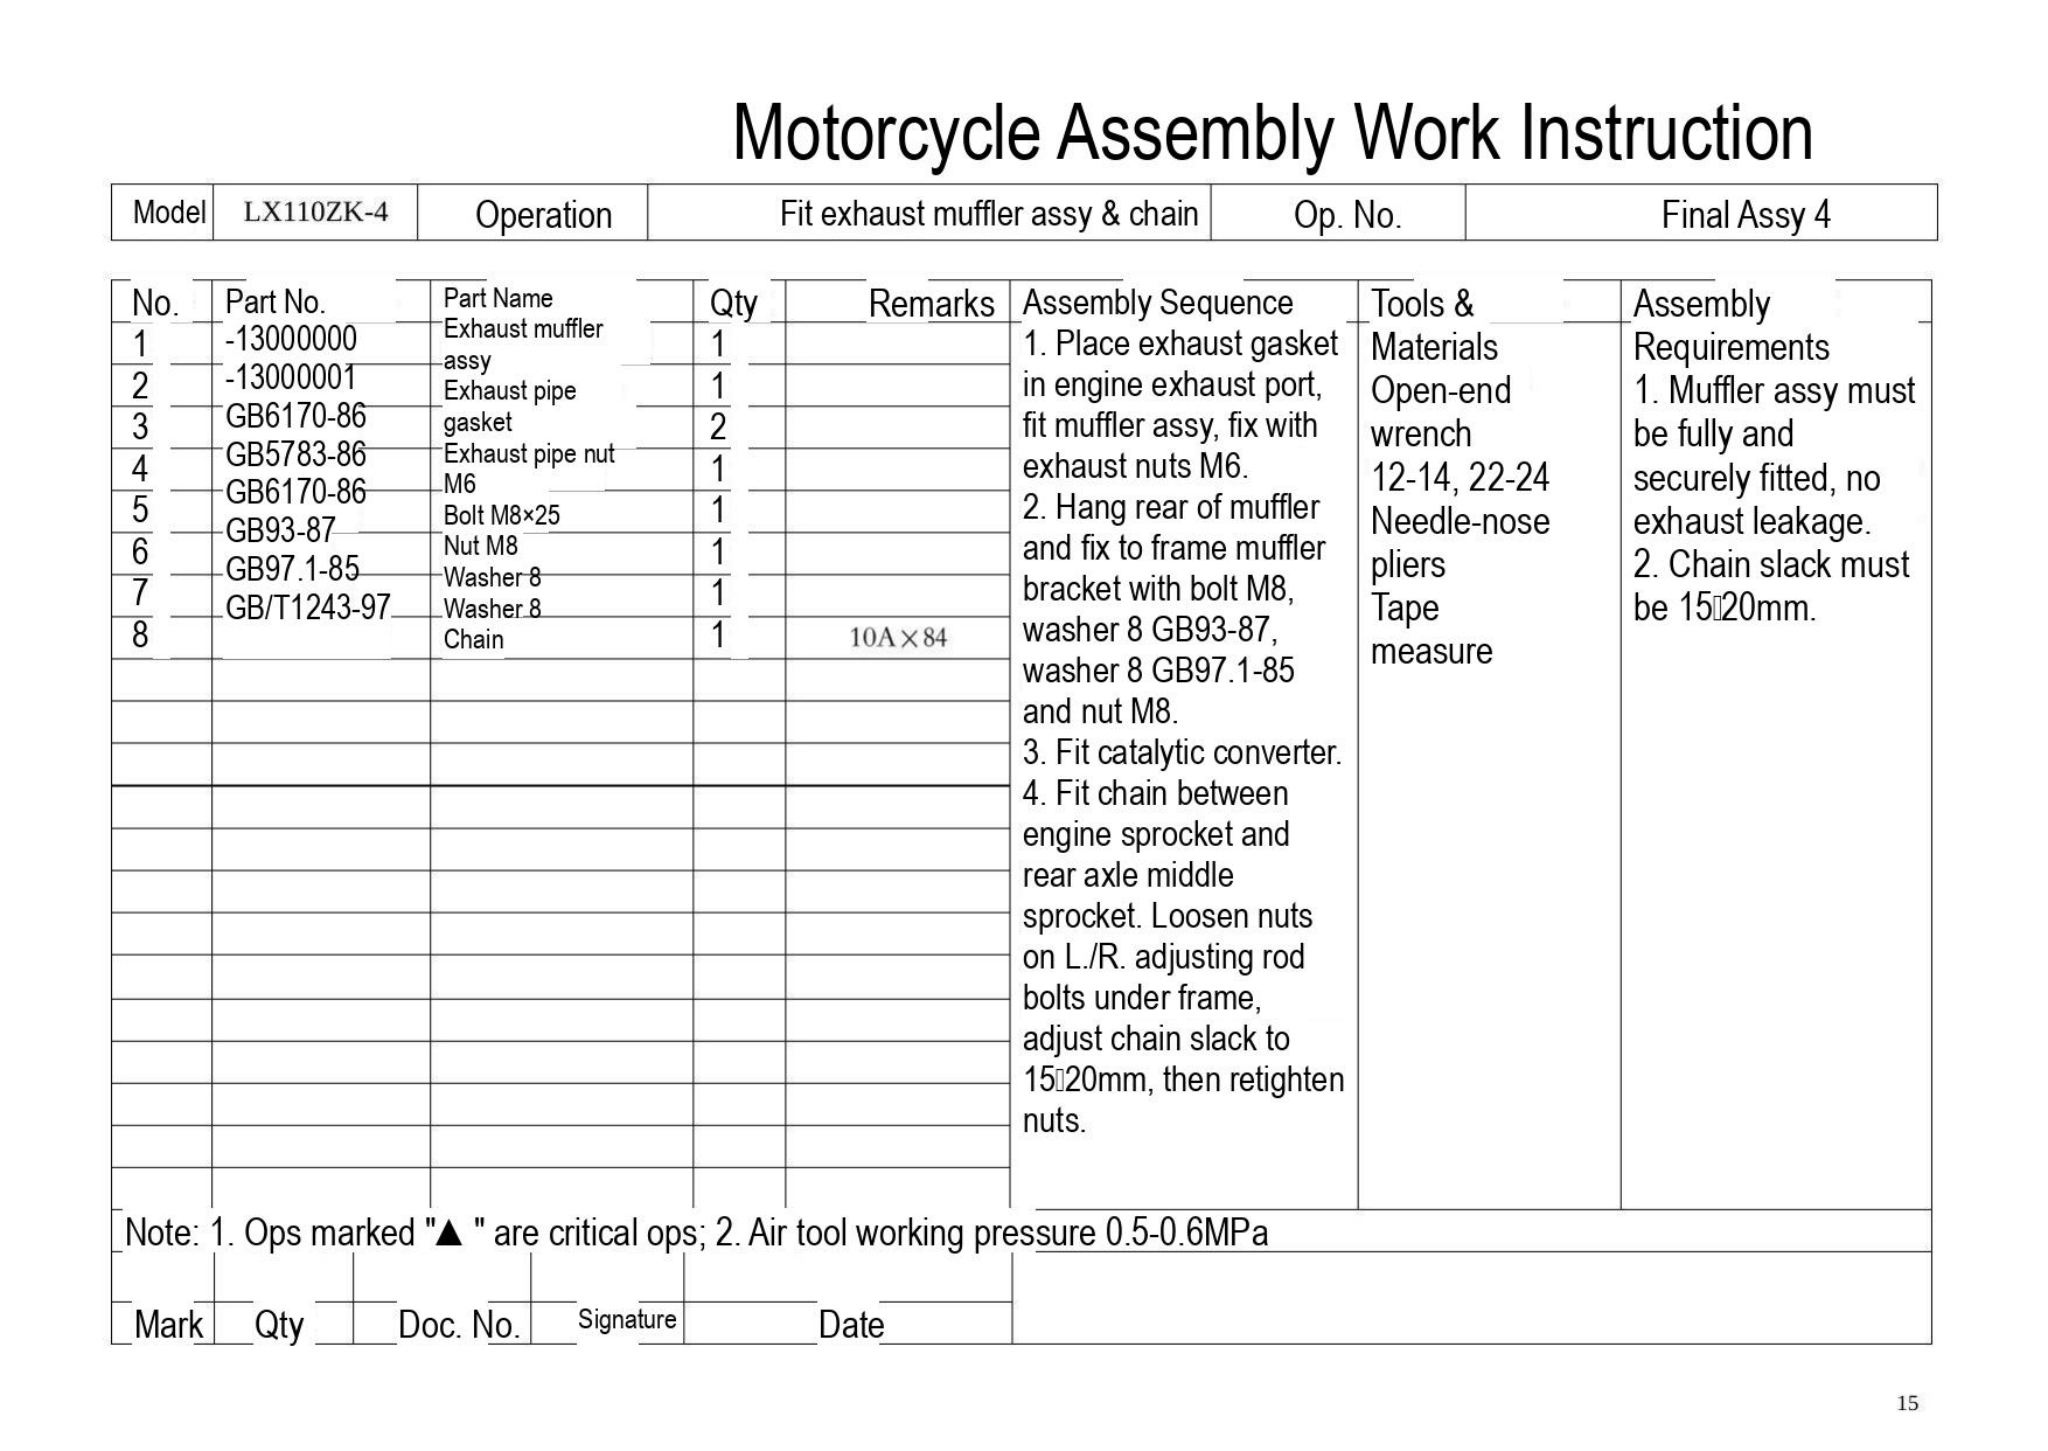# Motorcycle Assembly Work Instruction

| Model | LX110ZK-4 | Operation | Fit exhaust muffler assy & chain | Op. No. | Final Assy 4 |
|---|---|---|---|---|---|

| No. | Part No. | Part Name | Qty | Remarks |
|---|---|---|---|---|
| 1 | -13000000 | Exhaust muffler assy | 1 | |
| 2 | -13000001 | Exhaust pipe gasket | 1 | |
| 3 | GB6170-86 | Exhaust pipe nut M6 | 2 | |
| 4 | GB5783-86 | Bolt M8×25 | 1 | |
| 5 | GB6170-86 | Nut M8 | 1 | |
| 6 | GB93-87 | Washer 8 | 1 | |
| 7 | GB97.1-85 | Washer 8 | 1 | |
| 8 | GB/T1243-97 | Chain | 1 | 10A×84 |

| Assembly Sequence | Tools & Materials | Assembly Requirements |
|---|---|---|
| 1. Place exhaust gasket in engine exhaust port, fit muffler assy, fix with exhaust nuts M6.<br>2. Hang rear of muffler and fix to frame muffler bracket with bolt M8, washer 8 GB93-87, washer 8 GB97.1-85 and nut M8.<br>3. Fit catalytic converter.<br>4. Fit chain between engine sprocket and rear axle middle sprocket. Loosen nuts on L./R. adjusting rod bolts under frame, adjust chain slack to 15▯20mm, then retighten nuts. | Open-end wrench 12-14, 22-24<br>Needle-nose pliers<br>Tape measure | 1. Muffler assy must be fully and securely fitted, no exhaust leakage.<br>2. Chain slack must be 15▯20mm. |

Note: 1. Ops marked "▲ " are critical ops; 2. Air tool working pressure 0.5-0.6MPa

| Mark | Qty | Doc. No. | Signature | Date |
|---|---|---|---|---|

15
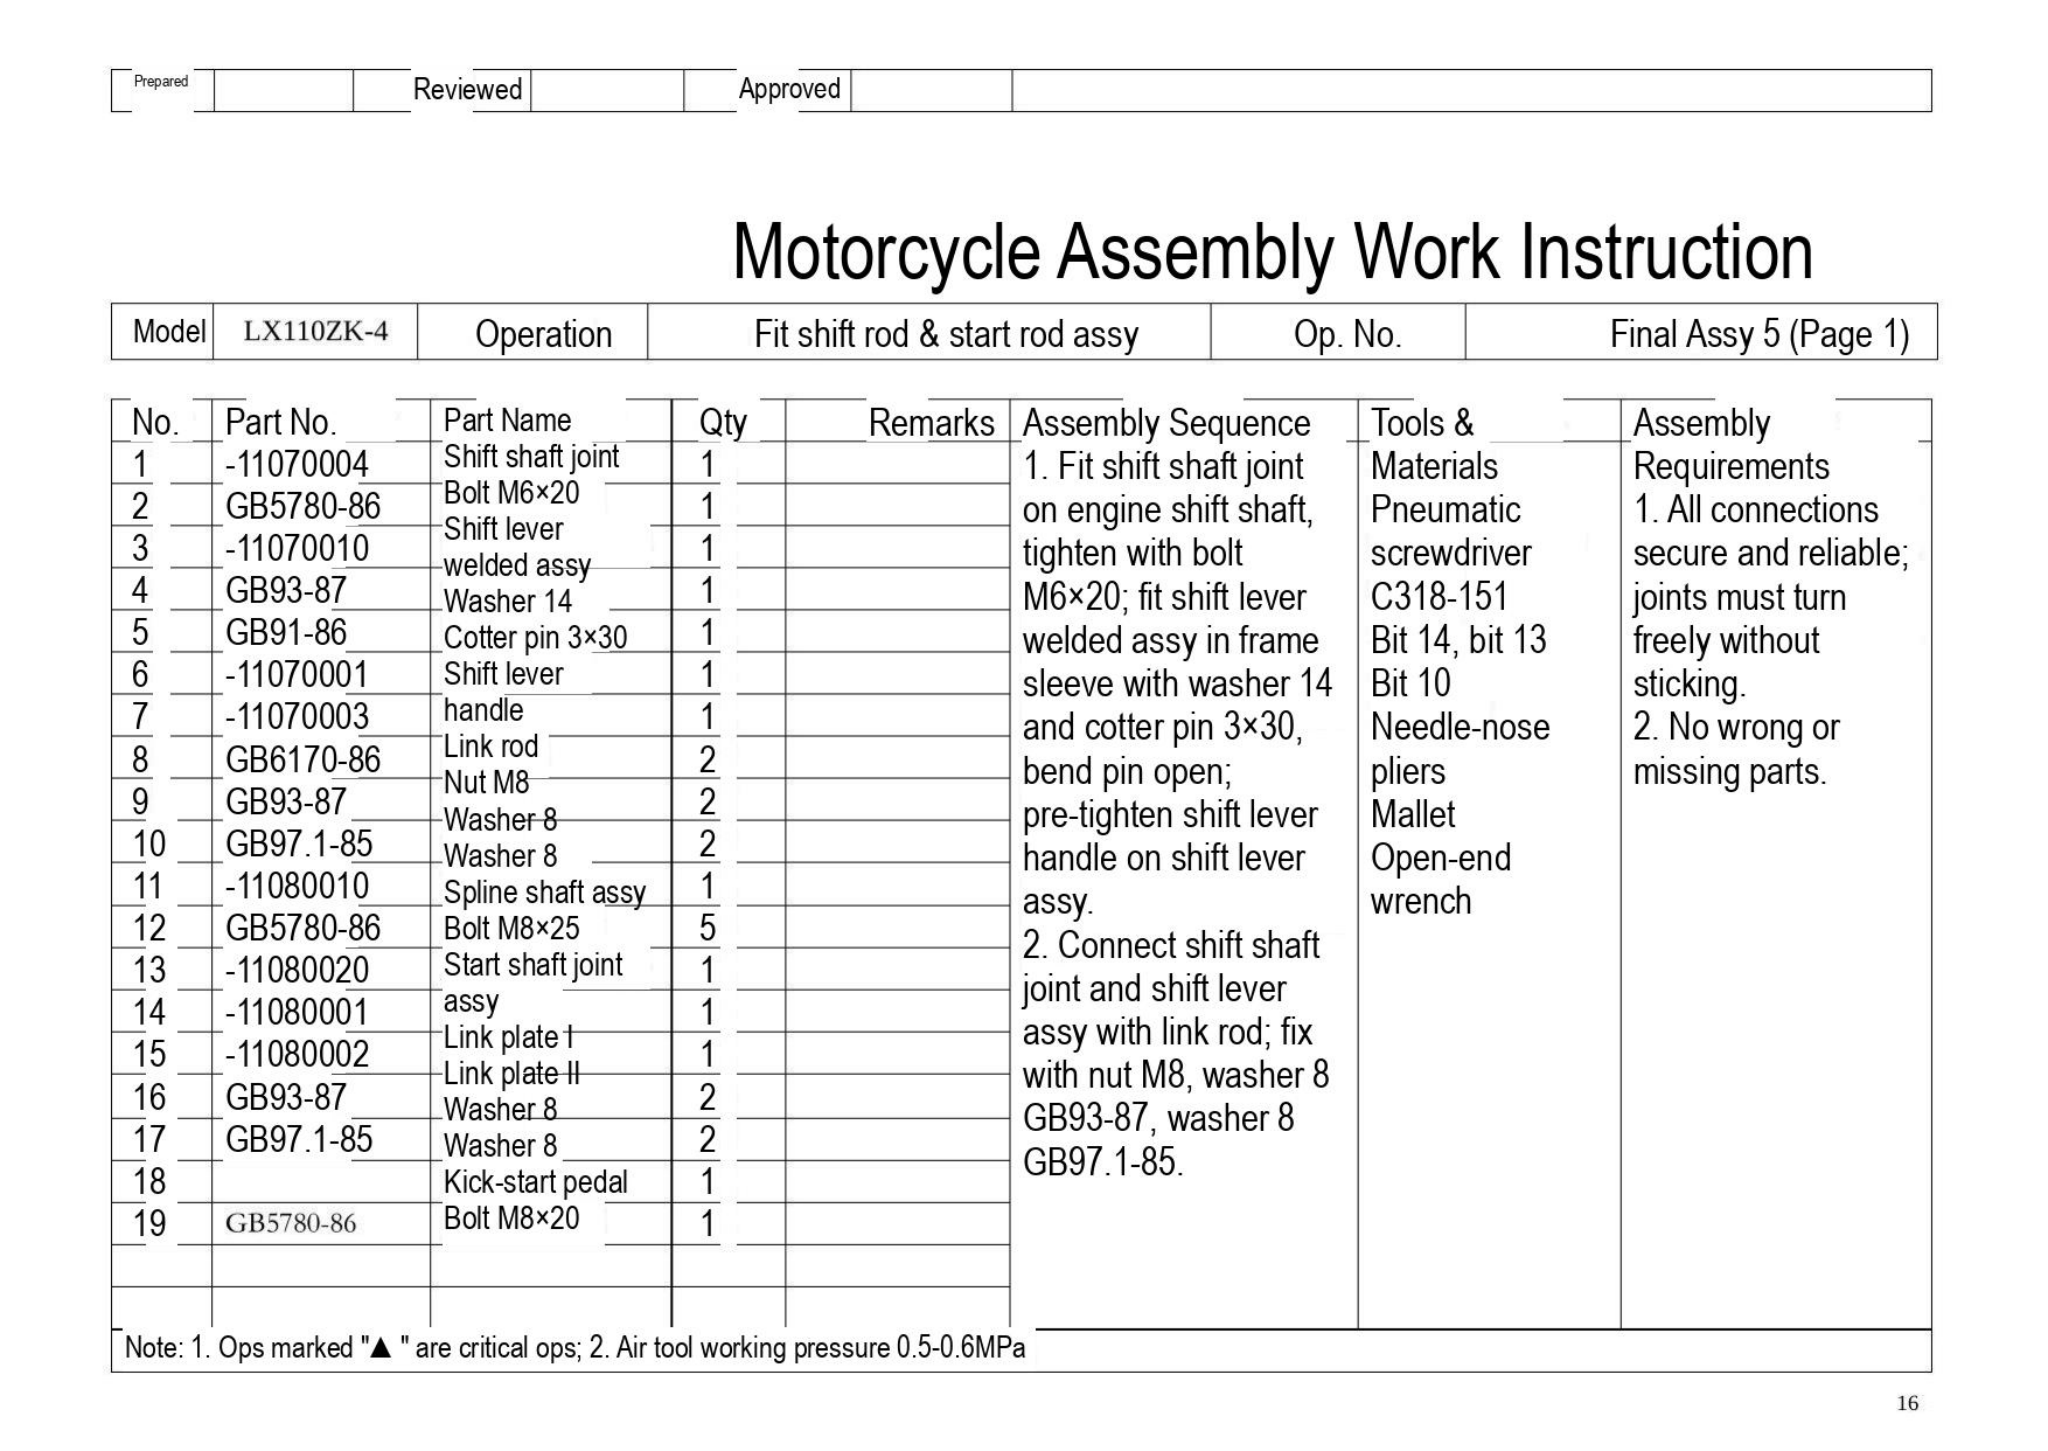| Prepared | | Reviewed | | Approved | | |
|---|---|---|---|---|---|---|

# Motorcycle Assembly Work Instruction

| Model | LX110ZK-4 | Operation | Fit shift rod & start rod assy | Op. No. | Final Assy 5 (Page 1) |
|---|---|---|---|---|---|

| No. | Part No. | Part Name | Qty | Remarks |
|---|---|---|---|---|
| 1 | -11070004 | Shift shaft joint | 1 | |
| 2 | GB5780-86 | Bolt M6×20 | 1 | |
| 3 | -11070010 | Shift lever welded assy | 1 | |
| 4 | GB93-87 | Washer 14 | 1 | |
| 5 | GB91-86 | Cotter pin 3×30 | 1 | |
| 6 | -11070001 | Shift lever handle | 1 | |
| 7 | -11070003 | Link rod | 1 | |
| 8 | GB6170-86 | Nut M8 | 2 | |
| 9 | GB93-87 | Washer 8 | 2 | |
| 10 | GB97.1-85 | Washer 8 | 2 | |
| 11 | -11080010 | Spline shaft assy | 1 | |
| 12 | GB5780-86 | Bolt M8×25 | 5 | |
| 13 | -11080020 | Start shaft joint assy | 1 | |
| 14 | -11080001 | Link plate I | 1 | |
| 15 | -11080002 | Link plate II | 1 | |
| 16 | GB93-87 | Washer 8 | 2 | |
| 17 | GB97.1-85 | Washer 8 | 2 | |
| 18 | | Kick-start pedal | 1 | |
| 19 | GB5780-86 | Bolt M8×20 | 1 | |
| | | | | |
| | | | | |

| Assembly Sequence | Tools & Materials | Assembly Requirements |
|---|---|---|
| 1. Fit shift shaft joint on engine shift shaft, tighten with bolt M6×20; fit shift lever welded assy in frame sleeve with washer 14 and cotter pin 3×30, bend pin open; pre-tighten shift lever handle on shift lever assy.<br>2. Connect shift shaft joint and shift lever assy with link rod; fix with nut M8, washer 8 GB93-87, washer 8 GB97.1-85. | Pneumatic screwdriver C318-151<br>Bit 14, bit 13<br>Bit 10<br>Needle-nose pliers<br>Mallet<br>Open-end wrench | 1. All connections secure and reliable; joints must turn freely without sticking.<br>2. No wrong or missing parts. |

Note: 1. Ops marked "▲ " are critical ops; 2. Air tool working pressure 0.5-0.6MPa

16
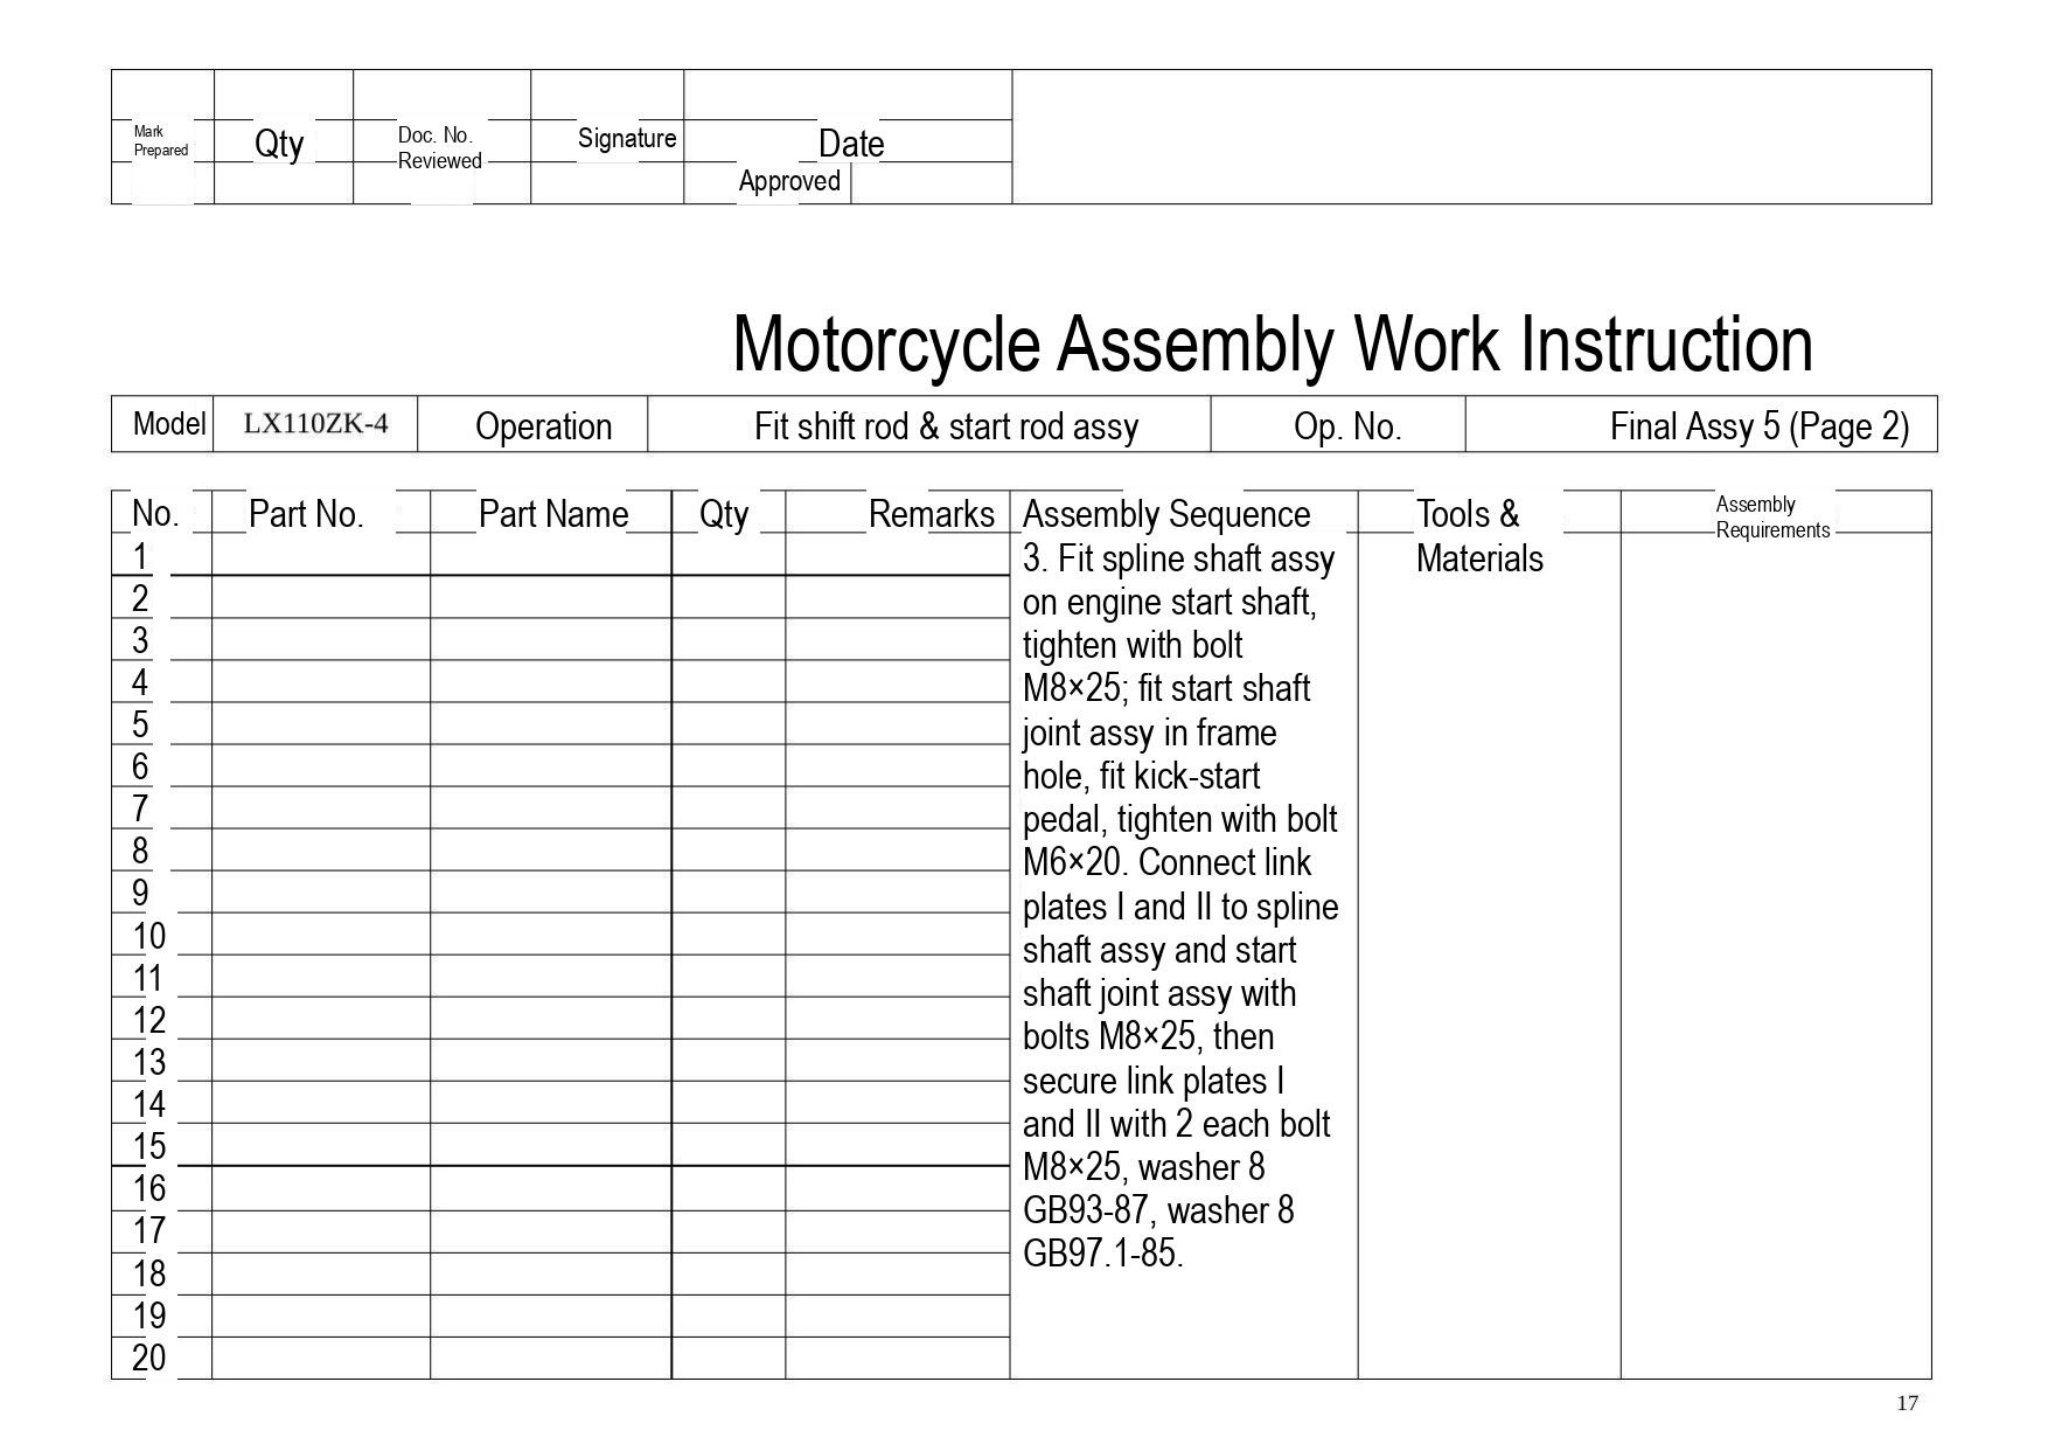| Mark Prepared | Qty | Doc. No. Reviewed | Signature | Date Approved |
|---|---|---|---|---|

# Motorcycle Assembly Work Instruction

| Model | LX110ZK-4 | Operation | Fit shift rod & start rod assy | Op. No. | Final Assy 5 (Page 2) |
|---|---|---|---|---|---|

| No. | Part No. | Part Name | Qty | Remarks | Assembly Sequence | Tools & Materials | Assembly Requirements |
|---|---|---|---|---|---|---|---|
| 1 | | | | | 3. Fit spline shaft assy on engine start shaft, tighten with bolt M8×25; fit start shaft joint assy in frame hole, fit kick-start pedal, tighten with bolt M6×20. Connect link plates I and II to spline shaft assy and start shaft joint assy with bolts M8×25, then secure link plates I and II with 2 each bolt M8×25, washer 8 GB93-87, washer 8 GB97.1-85. | | |
| 2 | | | | | | | |
| 3 | | | | | | | |
| 4 | | | | | | | |
| 5 | | | | | | | |
| 6 | | | | | | | |
| 7 | | | | | | | |
| 8 | | | | | | | |
| 9 | | | | | | | |
| 10 | | | | | | | |
| 11 | | | | | | | |
| 12 | | | | | | | |
| 13 | | | | | | | |
| 14 | | | | | | | |
| 15 | | | | | | | |
| 16 | | | | | | | |
| 17 | | | | | | | |
| 18 | | | | | | | |
| 19 | | | | | | | |
| 20 | | | | | | | |

17
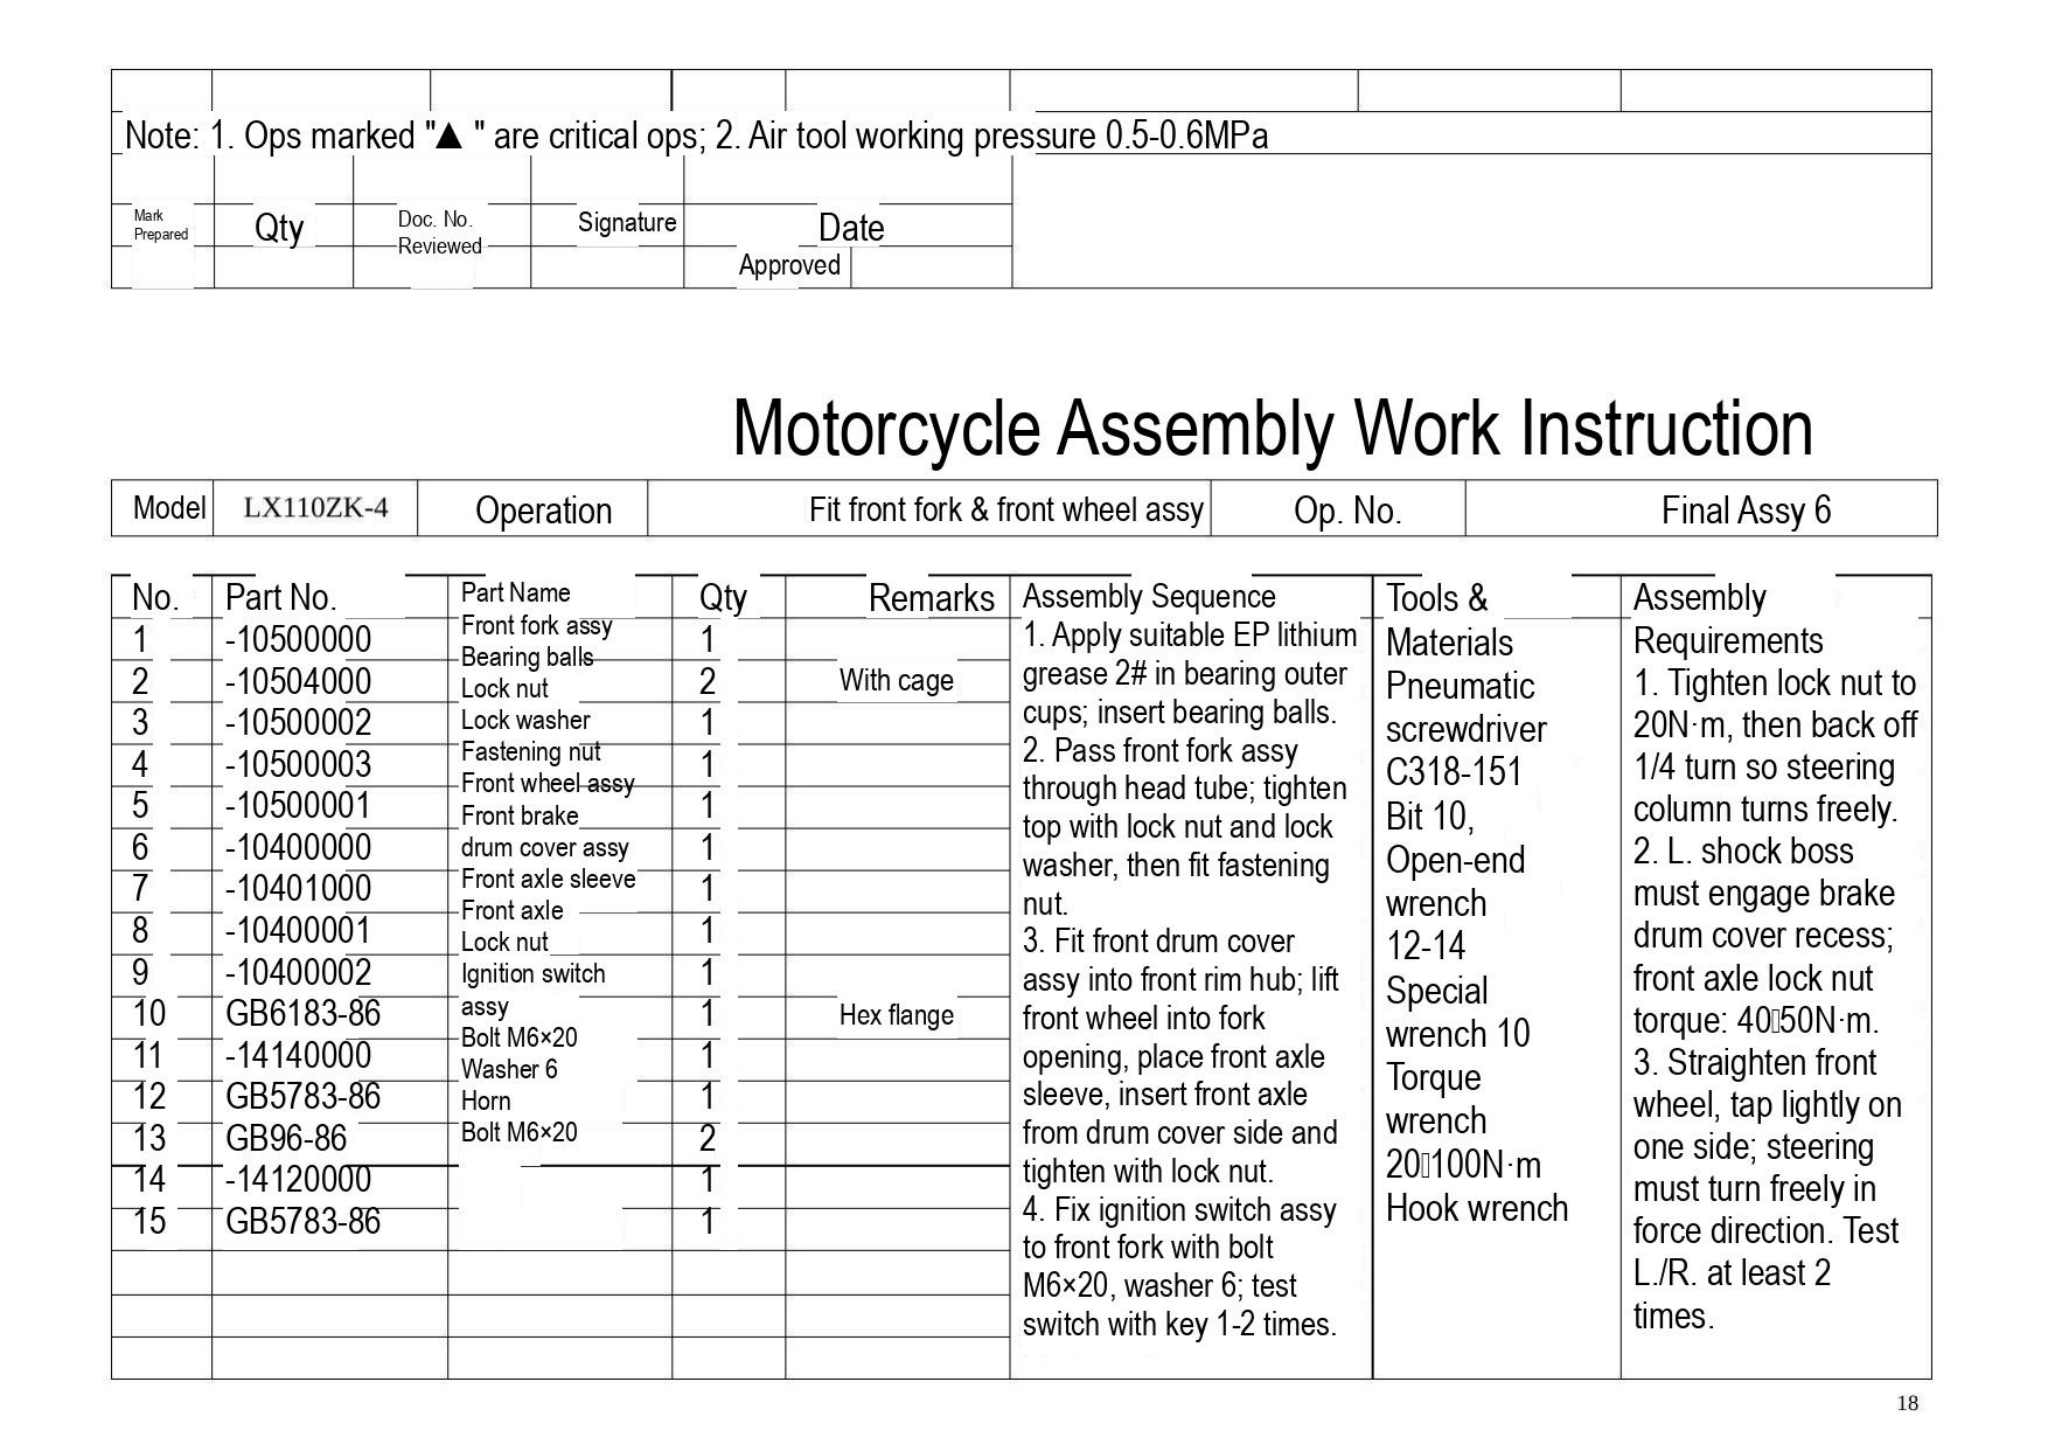Note: 1. Ops marked "▲ " are critical ops; 2. Air tool working pressure 0.5-0.6MPa

| Mark Prepared | Qty | Doc. No. Reviewed | Signature | Date | Approved |
|---|---|---|---|---|---|
| | | | | | |

# Motorcycle Assembly Work Instruction

| Model | LX110ZK-4 | Operation | Fit front fork & front wheel assy | Op. No. | Final Assy 6 |
|---|---|---|---|---|---|

| No. | Part No. | Part Name | Qty | Remarks |
|---|---|---|---|---|
| 1 | -10500000 | Front fork assy | 1 | |
| 2 | -10504000 | Bearing balls | 2 | With cage |
| 3 | -10500002 | Lock nut | 1 | |
| 4 | -10500003 | Lock washer | 1 | |
| 5 | -10500001 | Fastening nut | 1 | |
| 6 | -10400000 | Front wheel assy | 1 | |
| 7 | -10401000 | Front brake drum cover assy | 1 | |
| 8 | -10400001 | Front axle sleeve | 1 | |
| 9 | -10400002 | Front axle | 1 | |
| 10 | GB6183-86 | Lock nut | 1 | Hex flange |
| 11 | -14140000 | Ignition switch assy | 1 | |
| 12 | GB5783-86 | Bolt M6×20 | 1 | |
| 13 | GB96-86 | Washer 6 | 2 | |
| 14 | -14120000 | Horn | 1 | |
| 15 | GB5783-86 | Bolt M6×20 | 1 | |

**Assembly Sequence**
1. Apply suitable EP lithium grease 2# in bearing outer cups; insert bearing balls.
2. Pass front fork assy through head tube; tighten top with lock nut and lock washer, then fit fastening nut.
3. Fit front drum cover assy into front rim hub; lift front wheel into fork opening, place front axle sleeve, insert front axle from drum cover side and tighten with lock nut.
4. Fix ignition switch assy to front fork with bolt M6×20, washer 6; test switch with key 1-2 times.

**Tools & Materials**
Pneumatic screwdriver C318-151
Bit 10,
Open-end wrench 12-14
Special wrench 10
Torque wrench 20□100N·m
Hook wrench

**Assembly Requirements**
1. Tighten lock nut to 20N·m, then back off 1/4 turn so steering column turns freely.
2. L. shock boss must engage brake drum cover recess; front axle lock nut torque: 40□50N·m.
3. Straighten front wheel, tap lightly on one side; steering must turn freely in force direction. Test L./R. at least 2 times.

18
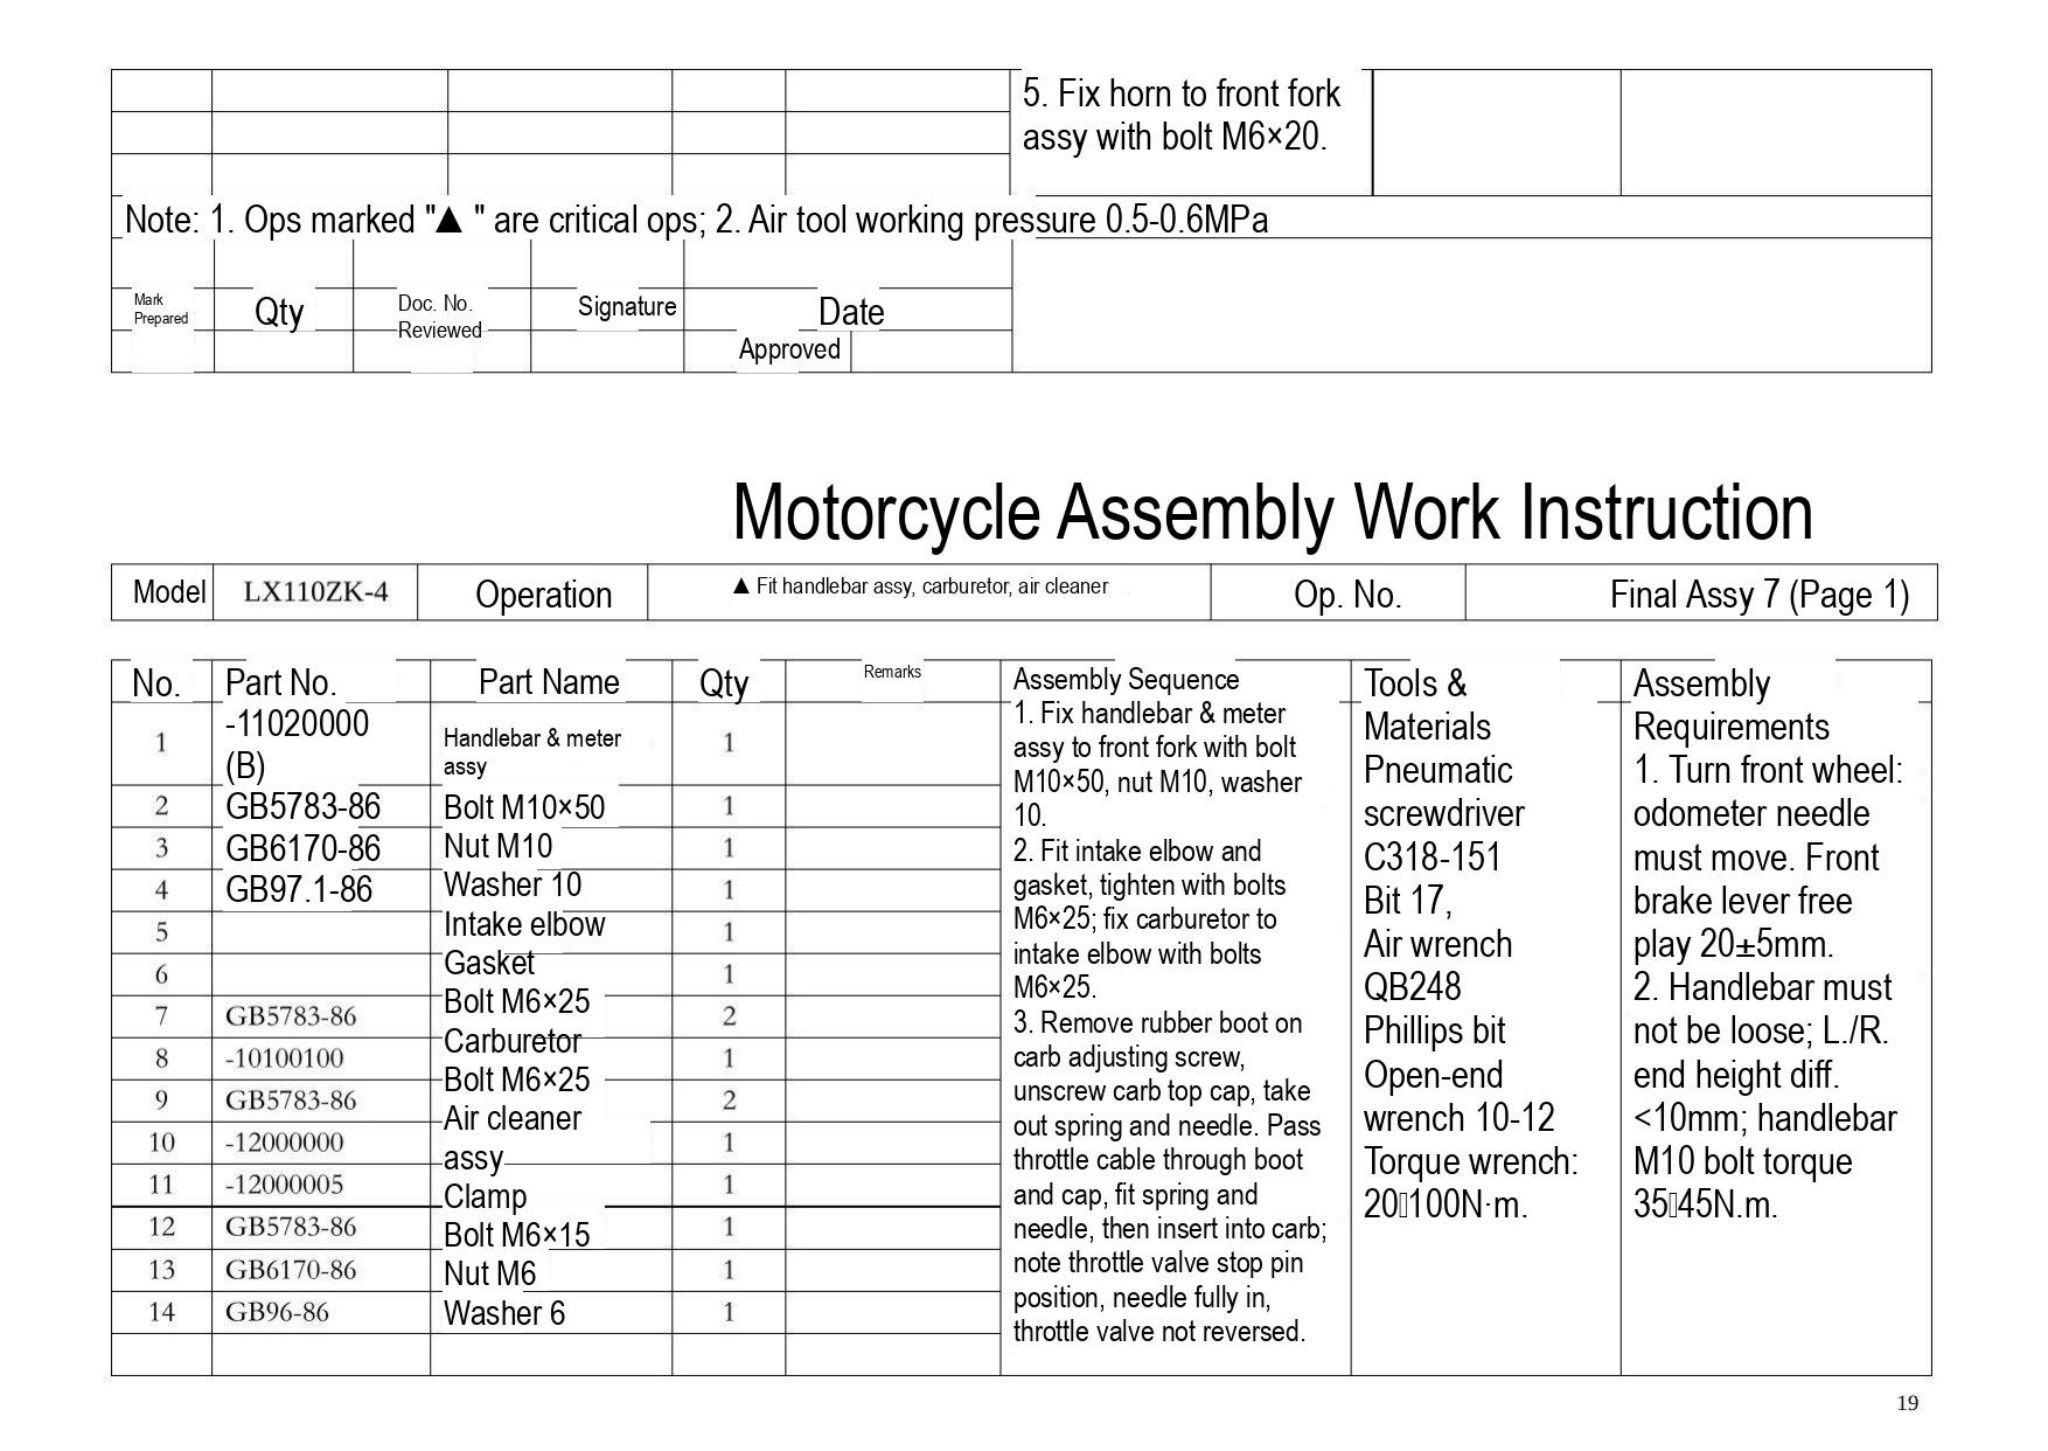5. Fix horn to front fork assy with bolt M6×20.

Note: 1. Ops marked "▲ " are critical ops; 2. Air tool working pressure 0.5-0.6MPa

| Mark Prepared | Qty | Doc. No. Reviewed | Signature | Date | Approved |
|---|---|---|---|---|---|

# Motorcycle Assembly Work Instruction

| Model | LX110ZK-4 | Operation | ▲ Fit handlebar assy, carburetor, air cleaner | Op. No. | Final Assy 7 (Page 1) |
|---|---|---|---|---|---|

| No. | Part No. | Part Name | Qty | Remarks | Assembly Sequence | Tools & Materials | Assembly Requirements |
|---|---|---|---|---|---|---|---|
| 1 | -11020000 (B) | Handlebar & meter assy | 1 | | 1. Fix handlebar & meter assy to front fork with bolt M10×50, nut M10, washer 10.<br>2. Fit intake elbow and gasket, tighten with bolts M6×25; fix carburetor to intake elbow with bolts M6×25.<br>3. Remove rubber boot on carb adjusting screw, unscrew carb top cap, take out spring and needle. Pass throttle cable through boot and cap, fit spring and needle, then insert into carb; note throttle valve stop pin position, needle fully in, throttle valve not reversed. | Pneumatic screwdriver C318-151<br>Bit 17,<br>Air wrench QB248<br>Phillips bit<br>Open-end wrench 10-12<br>Torque wrench: 20□100N·m. | 1. Turn front wheel: odometer needle must move. Front brake lever free play 20±5mm.<br>2. Handlebar must not be loose; L./R. end height diff. <10mm; handlebar M10 bolt torque 35□45N.m. |
| 2 | GB5783-86 | Bolt M10×50 | 1 | | | | |
| 3 | GB6170-86 | Nut M10 | 1 | | | | |
| 4 | GB97.1-86 | Washer 10 | 1 | | | | |
| 5 | | Intake elbow | 1 | | | | |
| 6 | | Gasket | 1 | | | | |
| 7 | GB5783-86 | Bolt M6×25 | 2 | | | | |
| 8 | -10100100 | Carburetor | 1 | | | | |
| 9 | GB5783-86 | Bolt M6×25 | 2 | | | | |
| 10 | -12000000 | Air cleaner assy | 1 | | | | |
| 11 | -12000005 | Clamp | 1 | | | | |
| 12 | GB5783-86 | Bolt M6×15 | 1 | | | | |
| 13 | GB6170-86 | Nut M6 | 1 | | | | |
| 14 | GB96-86 | Washer 6 | 1 | | | | |

19
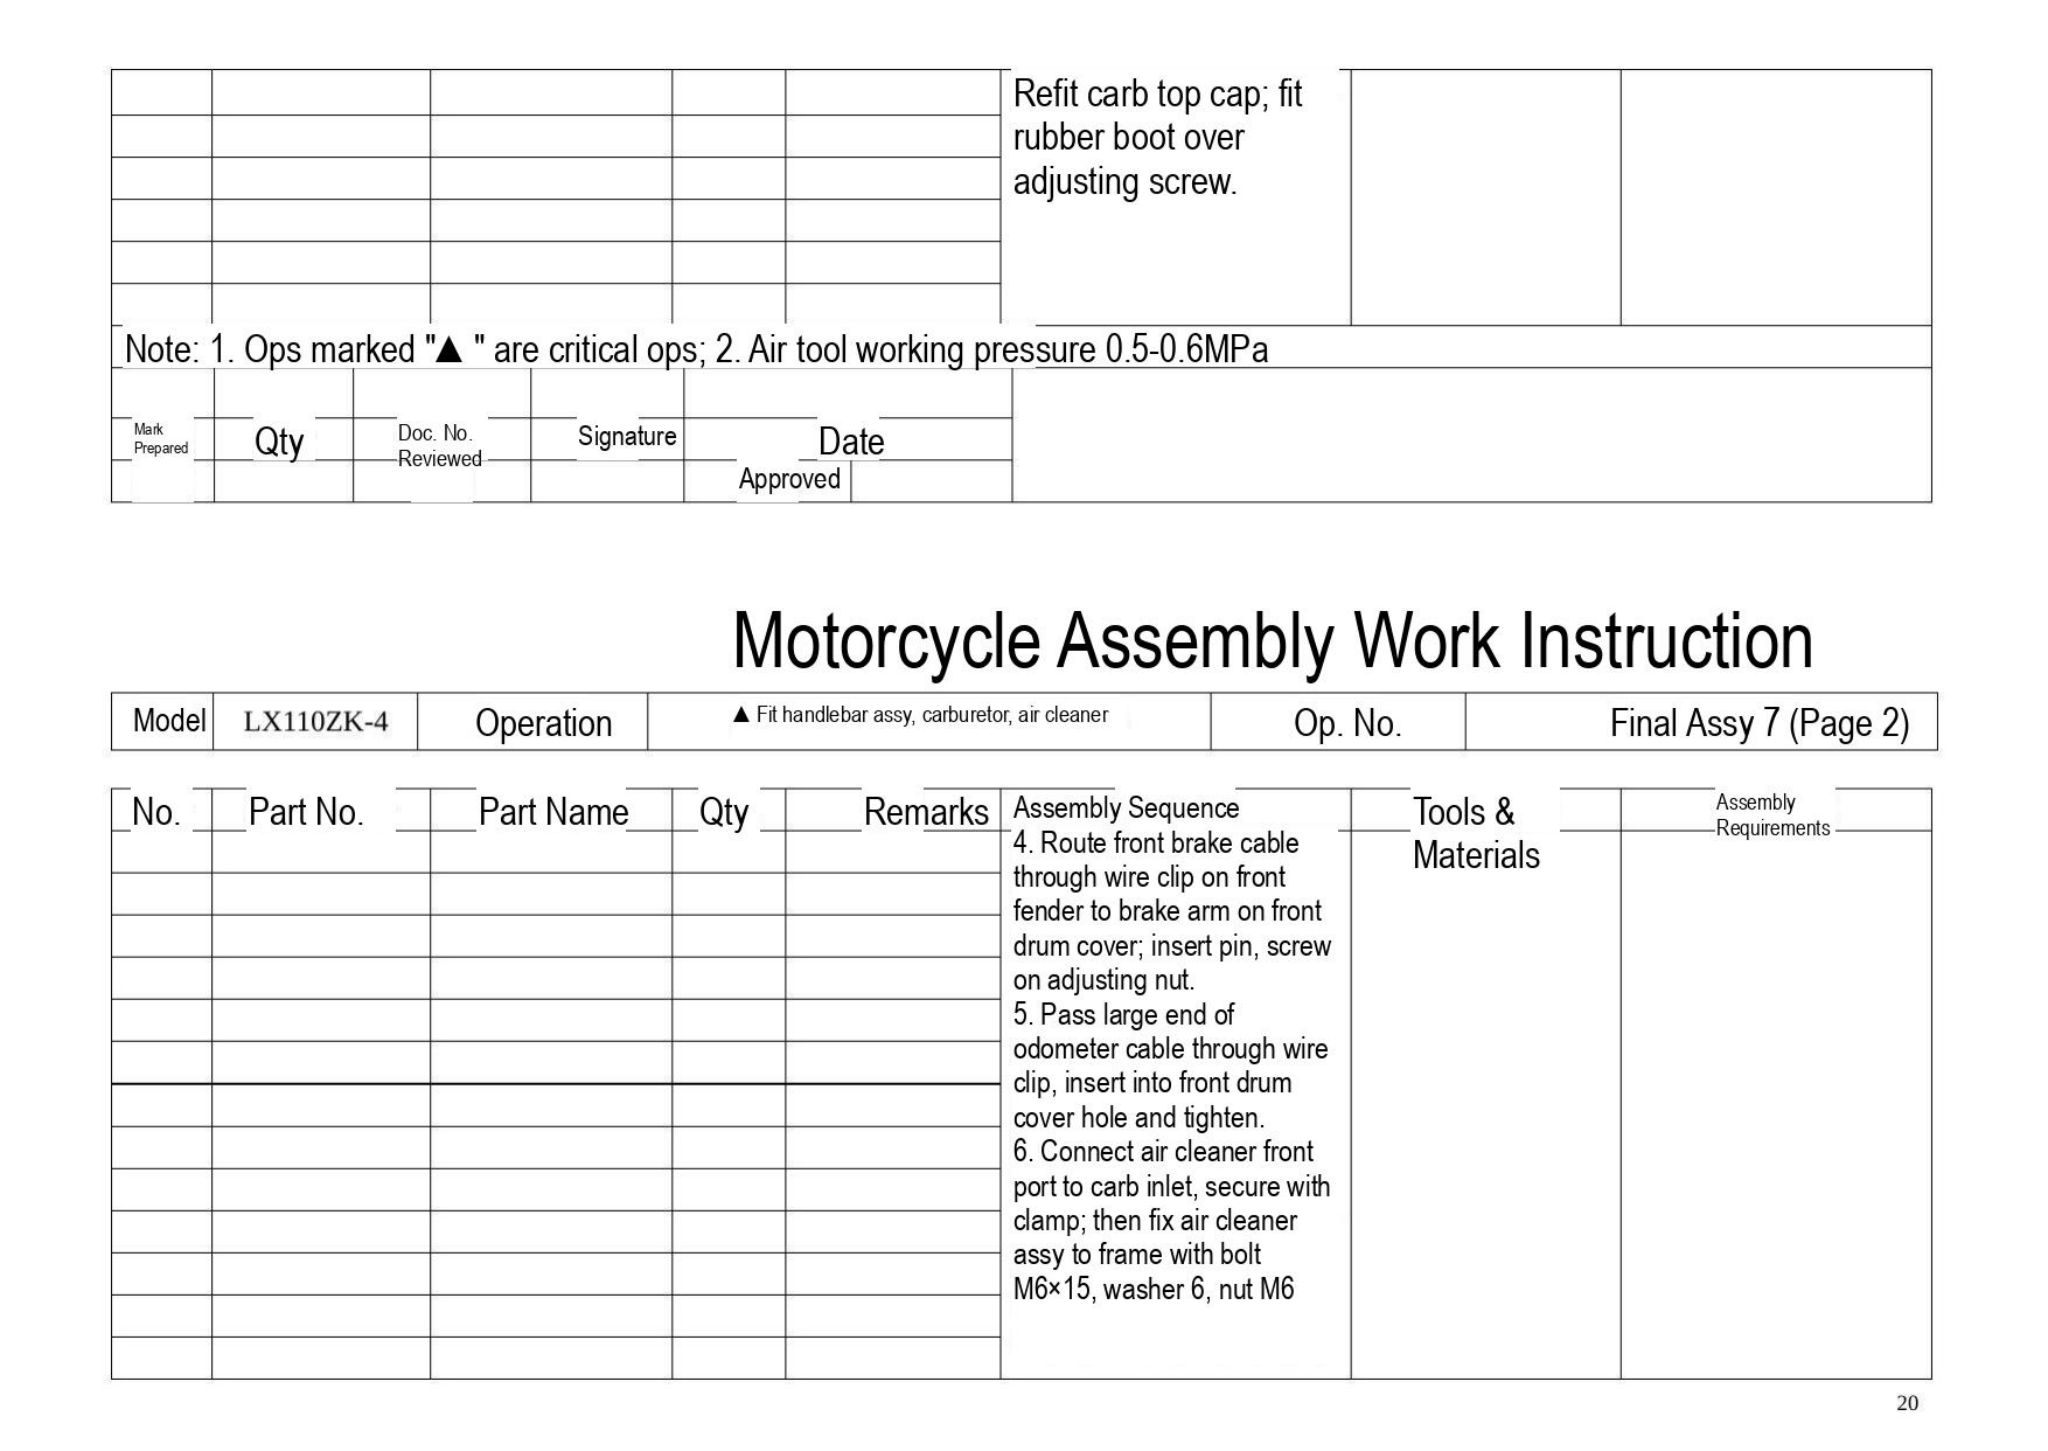Refit carb top cap; fit rubber boot over adjusting screw.

Note: 1. Ops marked "▲ " are critical ops; 2. Air tool working pressure 0.5-0.6MPa

| Mark Prepared | Qty | Doc. No. Reviewed | Signature | Date Approved |
|---|---|---|---|---|

# Motorcycle Assembly Work Instruction

| Model | LX110ZK-4 | Operation | ▲ Fit handlebar assy, carburetor, air cleaner | Op. No. | Final Assy 7 (Page 2) |
|---|---|---|---|---|---|

| No. | Part No. | Part Name | Qty | Remarks | Assembly Sequence | Tools & Materials | Assembly Requirements |
|---|---|---|---|---|---|---|---|
| | | | | | 4. Route front brake cable through wire clip on front fender to brake arm on front drum cover; insert pin, screw on adjusting nut.<br>5. Pass large end of odometer cable through wire clip, insert into front drum cover hole and tighten.<br>6. Connect air cleaner front port to carb inlet, secure with clamp; then fix air cleaner assy to frame with bolt M6×15, washer 6, nut M6 | | |

20